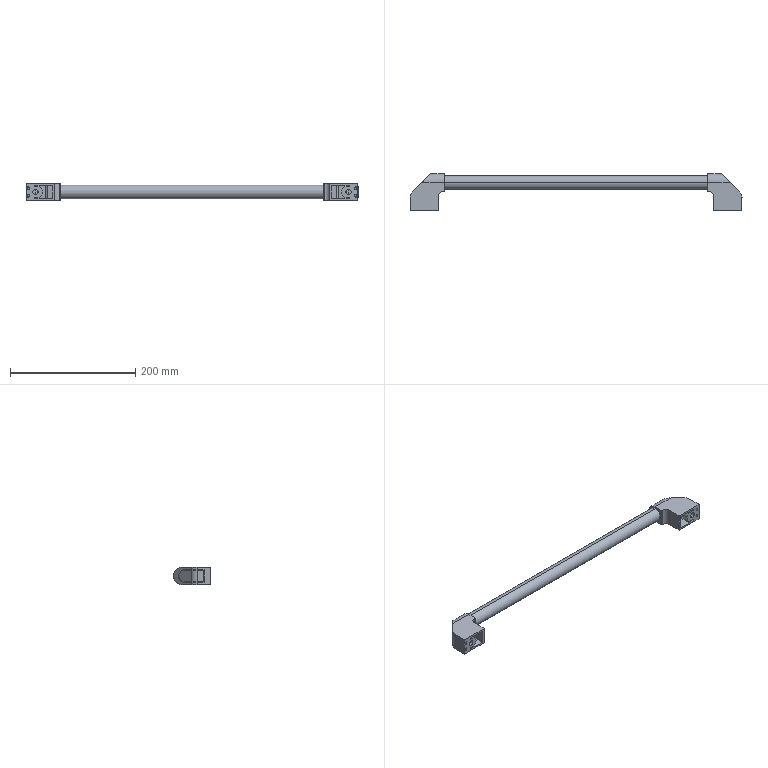Part | SolidWorks | features BaseBody 1 | 1 solid | 154 faces | box 530 x 58.6 x 28 mm | volume 258002 mm3 | plane 94 | cylinder 56 | cone 4 | commonest cylinder face diameters 1.2 x16 24 x6 2 x4 2.02 x4 8.5 x4 16.2 x4